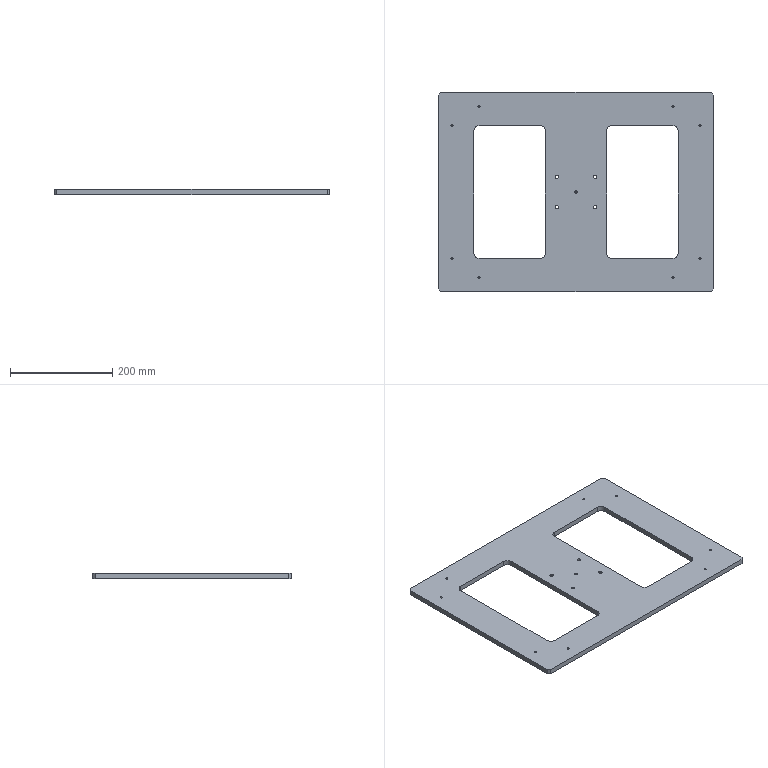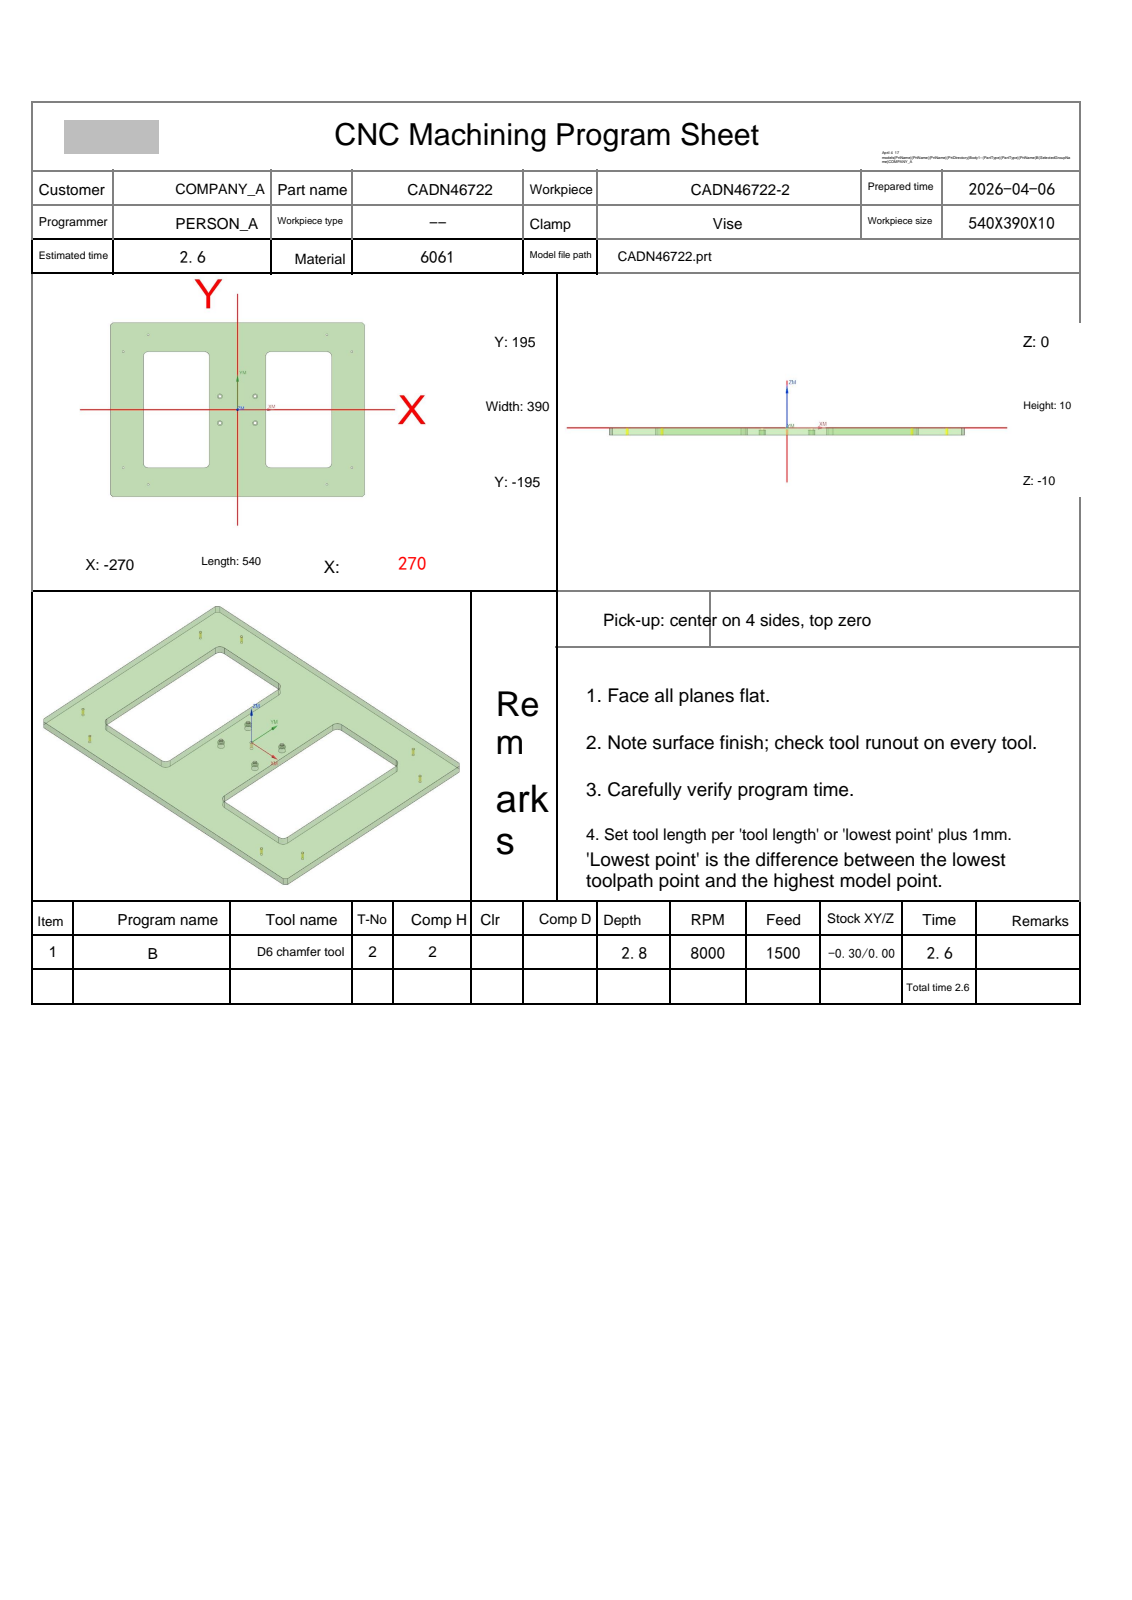NC program | NX | posted by the shop | part box 540 x 390 x 10 mm
Whole program:
%
O0001
(Machine time: 2.83 MIN)
(===Total Tool:1===)
(T2=D6 chamfer tool   D=6.   R=0.   D-  H02 Z=-2.8  )
G80 G90 G17 G49 G40
G91 G28 Z0
M01
N1 T02 M06
(D6 chamfer tool  D=6. R=0. H=02 ce=0.00 di=0.00)
G00 G90 G54 X-190. Y168. M03 S8000
G43 H02 Z20.
M08
G98 G81 X-190. Y168. Z-2.367 R3. F1000.
X-243. Y130.
Y-130.
X-190. Y-168.
X190.
X243. Y-130.
Y130.
X190. Y168.
G80
G00 Z20.
G00 G90 X0.0 Y0.0 M03 S8000
Z20.
G98 G81 X0.0 Y0.0 Z-2.8 R3. F1000.
G80
G00 Z20.
G00 G90 X-194.756 Y127.989 M03 S7000
Z20.
Z2.5
G01 X-195.084 Y127.791 Z2.361 F1500.
X-195.609 Y127.422 Z2.127
X-196.108 Y127.017 Z1.893
X-196.578 Y126.578 Z1.659
X-197.017 Y126.108 Z1.425
X-197.422 Y125.609 Z1.191
X-197.791 Y125.084 Z.957
X-198.124 Y124.534 Z.723
X-198.417 Y123.962 Z.489
X-198.671 Y123.371 Z.255
X-198.883 Y122.765 Z.022
X-199.052 Y122.145 Z-.212
X-199.179 Y121.515 Z-.446
X-199.262 Y120.878 Z-.68
X-199.3 Y120.236 Z-.914
Y120. Z-1.
Y-120.
G03 X-190. Y-129.3 I9.3 J0.0
G01 X-70.
G03 X-60.7 Y-120. I0.0 J9.3
G01 Y120.
G03 X-70. Y129.3 I-9.3 J0.0
G01 X-190.
G03 X-199.3 Y120. I0.0 J-9.3
G01 Y119.5
Z1.5
G00 Z20.
X-270.7 Y188.655
Z2.5
G01 Y189.876 Z2.056
Y189.953 Z2.027
X-270.662 Y190.16 Z1.951
X-270.581 Y190.355 Z1.874
X-270.462 Y190.528 Z1.798
X-265.528 Y195.462 Z-.742
X-265.355 Y195.581 Z-.819
X-265.16 Y195.662 Z-.895
X-264.953 Y195.7 Z-.972
X-264.876 Z-1.
X264.876
G02 X265.583 Y195.407 I0.0 J-1.
G01 X270.407 Y190.583
G02 X270.7 Y189.876 I-.707 J-.707
G01 Y-189.876
G02 X270.407 Y-190.583 I-1. J0.0
G01 X265.583 Y-195.407
G02 X264.876 Y-195.7 I-.707 J.707
G01 X-264.876
G02 X-265.583 Y-195.407 I0.0 J1.
G01 X-270.407 Y-190.583
G02 X-270.7 Y-189.876 I.707 J.707
G01 Y189.876
G02 X-270.407 Y190.583 I1. J0.0
G01 X-265.583 Y195.407
G02 X-264.876 Y195.7 I.707 J-.707
G01 X-264.376
Z1.5
G00 Z20.
X65.244 Y127.989
Z2.5
G01 X64.916 Y127.791 Z2.361
X64.391 Y127.422 Z2.127
X63.892 Y127.017 Z1.893
X63.422 Y126.578 Z1.659
X62.983 Y126.108 Z1.425
X62.578 Y125.609 Z1.191
X62.209 Y125.084 Z.957
X61.876 Y124.534 Z.723
X61.583 Y123.962 Z.489
X61.329 Y123.371 Z.255
X61.117 Y122.765 Z.022
X60.948 Y122.145 Z-.212
X60.821 Y121.515 Z-.446
X60.738 Y120.878 Z-.68
X60.7 Y120.236 Z-.914
Y120. Z-1.
Y-120.
G03 X70. Y-129.3 I9.3 J0.0
G01 X190.
G03 X199.3 Y-120. I0.0 J9.3
G01 Y120.
G03 X190. Y129.3 I-9.3 J0.0
G01 X70.
G03 X60.7 Y120. I0.0 J-9.3
G01 Y119.5
Z1.5
G00 Z20.
G00 G90 X-35.293 Y-31.37 M03 S7000
Z20.
Z2.5
G01 X-35.175 Y-31.17 Z2.416 F1500.
X-35.04 Y-30.851 Z2.29
X-34.949 Y-30.517 Z2.163
X-34.903 Y-30.173 Z2.037
Y-29.827 Z1.911
X-34.949 Y-29.483 Z1.785
X-35.04 Y-29.149 Z1.659
X-35.175 Y-28.83 Z1.533
X-35.351 Y-28.531 Z1.407
X-35.565 Y-28.259 Z1.281
X-35.813 Y-28.017 Z1.154
X-36.092 Y-27.811 Z1.028
X-36.308 Y-27.686 Z.937
X-36.626 Y-27.548 Z.811
X-36.96 Y-27.454 Z.685
X-37.303 Y-27.404 Z.559
X-37.649 Y-27.401 Z.433
X-37.993 Y-27.444 Z.307
X-38.328 Y-27.532 Z.181
X-38.649 Y-27.664 Z.054
X-38.949 Y-27.837 Z-.072
X-39.223 Y-28.049 Z-.198
X-39.467 Y-28.295 Z-.324
X-39.676 Y-28.572 Z-.45
X-39.846 Y-28.873 Z-.576
X-39.975 Y-29.195 Z-.702
X-40.06 Y-29.531 Z-.828
X-40.1 Y-29.875 Z-.955
Y-30. Z-1.
G03 X-37.5 Y-32.6 I2.6 J0.0
X-34.9 Y-30. I0.0 J2.6
X-37.5 Y-27.4 I-2.6 J0.0
X-40.1 Y-30. I0.0 J-2.6
X-40.052 Y-30.497 I2.6 J0.0
G01 Z1.5
G00 Z20.
X-35.293 Y28.63
Z2.5
G01 X-35.175 Y28.83 Z2.416
X-35.04 Y29.149 Z2.29
X-34.949 Y29.483 Z2.163
X-34.903 Y29.827 Z2.037
Y30.173 Z1.911
X-34.949 Y30.517 Z1.785
X-35.04 Y30.851 Z1.659
X-35.175 Y31.17 Z1.533
X-35.351 Y31.469 Z1.407
X-35.565 Y31.741 Z1.281
X-35.813 Y31.983 Z1.154
X-36.092 Y32.189 Z1.028
X-36.308 Y32.314 Z.937
X-36.626 Y32.452 Z.811
X-36.96 Y32.546 Z.685
X-37.303 Y32.596 Z.559
X-37.649 Y32.599 Z.433
X-37.993 Y32.556 Z.307
X-38.328 Y32.468 Z.181
X-38.649 Y32.336 Z.054
X-38.949 Y32.163 Z-.072
X-39.223 Y31.951 Z-.198
X-39.467 Y31.705 Z-.324
X-39.676 Y31.428 Z-.45
X-39.846 Y31.127 Z-.576
X-39.975 Y30.805 Z-.702
X-40.06 Y30.469 Z-.828
X-40.1 Y30.125 Z-.955
Y30. Z-1.
G03 X-37.5 Y27.4 I2.6 J0.0
X-34.9 Y30. I0.0 J2.6
X-37.5 Y32.6 I-2.6 J0.0
X-40.1 Y30. I0.0 J-2.6
X-40.052 Y29.503 I2.6 J0.0
G01 Z1.5
G00 Z20.
X39.707 Y28.63
Z2.5
G01 X39.825 Y28.83 Z2.416
X39.96 Y29.149 Z2.29
X40.051 Y29.483 Z2.163
X40.097 Y29.827 Z2.037
Y30.173 Z1.911
X40.051 Y30.517 Z1.785
X39.96 Y30.851 Z1.659
X39.825 Y31.17 Z1.533
X39.649 Y31.469 Z1.407
X39.435 Y31.741 Z1.281
X39.187 Y31.983 Z1.154
X38.908 Y32.189 Z1.028
X38.692 Y32.314 Z.937
X38.374 Y32.452 Z.811
X38.04 Y32.546 Z.685
X37.697 Y32.596 Z.559
X37.351 Y32.599 Z.433
X37.007 Y32.556 Z.307
X36.672 Y32.468 Z.181
X36.351 Y32.336 Z.054
X36.051 Y32.163 Z-.072
X35.777 Y31.951 Z-.198
X35.533 Y31.705 Z-.324
X35.324 Y31.428 Z-.45
X35.154 Y31.127 Z-.576
X35.025 Y30.805 Z-.702
X34.94 Y30.469 Z-.828
X34.9 Y30.125 Z-.955
Y30. Z-1.
G03 X37.5 Y27.4 I2.6 J0.0
X40.1 Y30. I0.0 J2.6
X37.5 Y32.6 I-2.6 J0.0
X34.9 Y30. I0.0 J-2.6
X34.948 Y29.503 I2.6 J0.0
G01 Z1.5
G00 Z20.
X39.707 Y-31.37
Z2.5
G01 X39.825 Y-31.17 Z2.416
X39.96 Y-30.851 Z2.29
X40.051 Y-30.517 Z2.163
X40.097 Y-30.173 Z2.037
Y-29.827 Z1.911
X40.051 Y-29.483 Z1.785
X39.96 Y-29.149 Z1.659
X39.825 Y-28.83 Z1.533
X39.649 Y-28.531 Z1.407
X39.435 Y-28.259 Z1.281
X39.187 Y-28.017 Z1.154
X38.908 Y-27.811 Z1.028
X38.692 Y-27.686 Z.937
X38.374 Y-27.548 Z.811
X38.04 Y-27.454 Z.685
X37.697 Y-27.404 Z.559
X37.351 Y-27.401 Z.433
X37.007 Y-27.444 Z.307
X36.672 Y-27.532 Z.181
X36.351 Y-27.664 Z.054
X36.051 Y-27.837 Z-.072
X35.777 Y-28.049 Z-.198
X35.533 Y-28.295 Z-.324
X35.324 Y-28.572 Z-.45
X35.154 Y-28.873 Z-.576
X35.025 Y-29.195 Z-.702
X34.94 Y-29.531 Z-.828
X34.9 Y-29.875 Z-.955
Y-30. Z-1.
G03 X37.5 Y-32.6 I2.6 J0.0
X40.1 Y-30. I0.0 J2.6
X37.5 Y-27.4 I-2.6 J0.0
X34.9 Y-30. I0.0 J-2.6
X34.948 Y-30.497 I2.6 J0.0
G01 Z1.5
G00 Z20.
M05
M09
G91 G28 Z0.0
G91 G28 Y0.0
M30
%